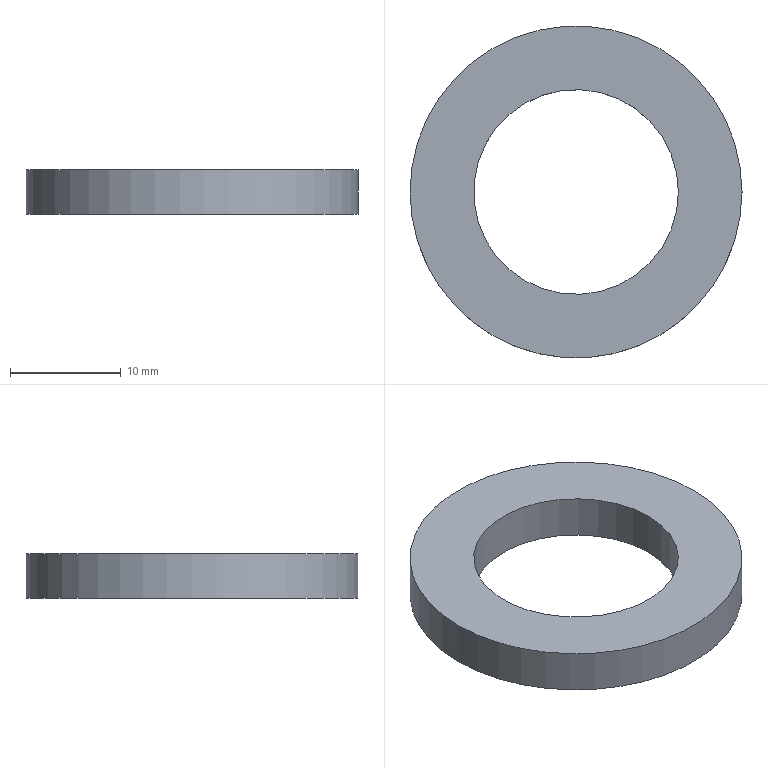Part | NX | features DATUM_CSYS 2, EXTRUDE 1, SKETCH 1 | 1 solid | 4 faces | box 30 x 30 x 4 mm | volume 1752 mm3 | cylinder 2 | plane 2 | commonest cylinder face diameters 18.5 x1 30 x1
STEP:
#1=CARTESIAN_POINT('',(15.,0.,-4.));
#2=VERTEX_POINT('',#1);
#3=CARTESIAN_POINT('',(0.,0.,-4.));
#4=DIRECTION('',(0.,0.,1.));
#5=DIRECTION('',(1.,0.,0.));
#6=AXIS2_PLACEMENT_3D('',#3,#4,#5);
#7=CIRCLE('',#6,15.);
#8=EDGE_CURVE('',#2,#2,#7,.T.);
#9=ORIENTED_EDGE('',*,*,#8,.T.);
#10=EDGE_LOOP('',(#9));
#11=FACE_BOUND('',#10,.T.);
#12=CARTESIAN_POINT('',(15.,0.,0.));
#13=VERTEX_POINT('',#12);
#14=CARTESIAN_POINT('',(0.,0.,0.));
#15=DIRECTION('',(0.,0.,1.));
#16=DIRECTION('',(1.,0.,0.));
#17=AXIS2_PLACEMENT_3D('',#14,#15,#16);
#18=CIRCLE('',#17,15.);
#19=EDGE_CURVE('',#13,#13,#18,.T.);
#20=ORIENTED_EDGE('',*,*,#19,.F.);
#21=EDGE_LOOP('',(#20));
#22=FACE_BOUND('',#21,.T.);
#23=CARTESIAN_POINT('',(0.,0.,-4.));
#24=DIRECTION('',(0.,0.,1.));
#25=DIRECTION('',(1.,0.,0.));
#26=AXIS2_PLACEMENT_3D('',#23,#24,#25);
#27=CYLINDRICAL_SURFACE('',#26,15.);
#28=ADVANCED_FACE('',(#11,#22),#27,.T.);
#29=CARTESIAN_POINT('',(9.25,0.,-4.));
#30=VERTEX_POINT('',#29);
#31=CARTESIAN_POINT('',(0.,0.,-4.));
#32=DIRECTION('',(0.,0.,1.));
#33=DIRECTION('',(1.,0.,0.));
#34=AXIS2_PLACEMENT_3D('',#31,#32,#33);
#35=CIRCLE('',#34,9.25);
#36=EDGE_CURVE('',#30,#30,#35,.T.);
#37=ORIENTED_EDGE('',*,*,#36,.F.);
#38=EDGE_LOOP('',(#37));
#39=FACE_BOUND('',#38,.T.);
#40=CARTESIAN_POINT('',(9.25,0.,0.));
#41=VERTEX_POINT('',#40);
#42=CARTESIAN_POINT('',(0.,0.,0.));
#43=DIRECTION('',(0.,0.,1.));
#44=DIRECTION('',(1.,0.,0.));
#45=AXIS2_PLACEMENT_3D('',#42,#43,#44);
#46=CIRCLE('',#45,9.25);
#47=EDGE_CURVE('',#41,#41,#46,.T.);
#48=ORIENTED_EDGE('',*,*,#47,.T.);
#49=EDGE_LOOP('',(#48));
#50=FACE_BOUND('',#49,.T.);
#51=CARTESIAN_POINT('',(0.,0.,-4.));
#52=DIRECTION('',(0.,0.,1.));
#53=DIRECTION('',(1.,0.,0.));
#54=AXIS2_PLACEMENT_3D('',#51,#52,#53);
#55=CYLINDRICAL_SURFACE('',#54,9.25);
#56=ADVANCED_FACE('',(#39,#50),#55,.F.);
#57=ORIENTED_EDGE('',*,*,#8,.F.);
#58=EDGE_LOOP('',(#57));
#59=FACE_BOUND('',#58,.T.);
#60=ORIENTED_EDGE('',*,*,#36,.T.);
#61=EDGE_LOOP('',(#60));
#62=FACE_BOUND('',#61,.T.);
#63=CARTESIAN_POINT('',(0.,0.,-4.));
#64=DIRECTION('',(0.,0.,1.));
#65=DIRECTION('',(1.,0.,0.));
#66=AXIS2_PLACEMENT_3D('',#63,#64,#65);
#67=PLANE('',#66);
#68=ADVANCED_FACE('',(#59,#62),#67,.F.);
#69=ORIENTED_EDGE('',*,*,#19,.T.);
#70=EDGE_LOOP('',(#69));
#71=FACE_BOUND('',#70,.T.);
#72=ORIENTED_EDGE('',*,*,#47,.F.);
#73=EDGE_LOOP('',(#72));
#74=FACE_BOUND('',#73,.T.);
#75=CARTESIAN_POINT('',(0.,0.,0.));
#76=DIRECTION('',(0.,0.,1.));
#77=DIRECTION('',(1.,0.,0.));
#78=AXIS2_PLACEMENT_3D('',#75,#76,#77);
#79=PLANE('',#78);
#80=ADVANCED_FACE('',(#71,#74),#79,.T.);
#81=CLOSED_SHELL('',(#28,#56,#68,#80));
#82=MANIFOLD_SOLID_BREP('',#81);
#83=(LENGTH_UNIT()NAMED_UNIT(*)SI_UNIT(.MILLI.,.METRE.));
#84=UNCERTAINTY_MEASURE_WITH_UNIT(LENGTH_MEASURE(0.00001),#83,'','');
#85=(NAMED_UNIT(*)PLANE_ANGLE_UNIT()SI_UNIT($,.RADIAN.));
#86=(NAMED_UNIT(*)SI_UNIT($,.STERADIAN.)SOLID_ANGLE_UNIT());
#87=(GEOMETRIC_REPRESENTATION_CONTEXT(3)GLOBAL_UNCERTAINTY_ASSIGNED_CONTEXT((#84))GLOBAL_UNIT_ASSIGNED_CONTEXT((#83,#85,#86))REPRESENTATION_CONTEXT('',''));
#88=ADVANCED_BREP_SHAPE_REPRESENTATION('',(#82),#87);